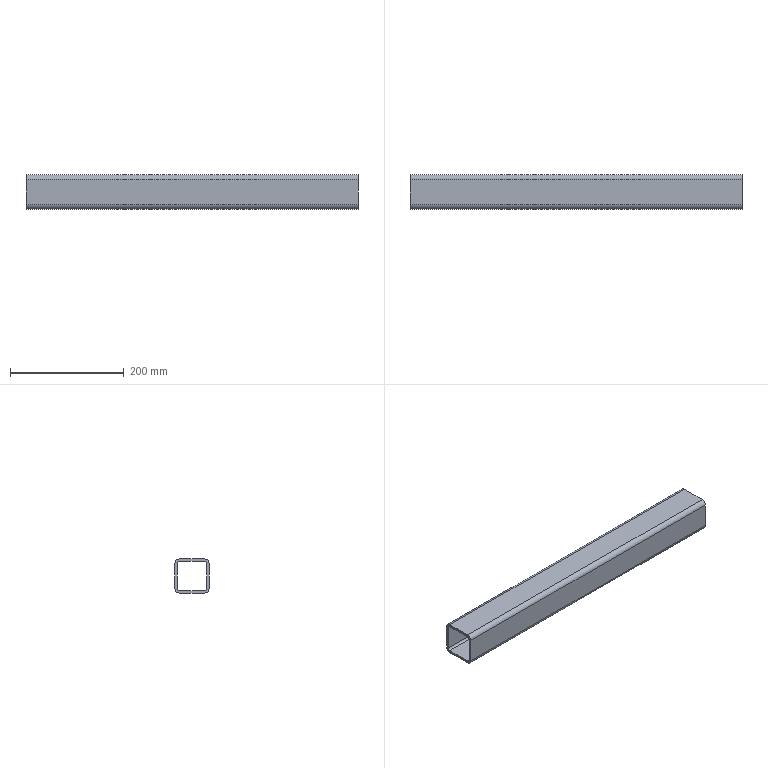Part | SolidWorks | features BaseBody 1 | 1 solid | 18 faces | box 585 x 60 x 60 mm | volume 500056 mm3 | plane 10 | cylinder 8 | commonest cylinder face diameters 8 x4 16 x4
STEP:
#1=CARTESIAN_POINT('',(-55.,2436.,-1248.));
#2=VERTEX_POINT('',#1);
#3=CARTESIAN_POINT('',(-55.,2436.,-1292.));
#4=VERTEX_POINT('',#3);
#5=CARTESIAN_POINT('',(-55.,2436.,-1248.));
#6=DIRECTION('',(0.,0.,-1.));
#7=VECTOR('',#6,1000.);
#8=LINE('',#5,#7);
#9=EDGE_CURVE('',#2,#4,#8,.T.);
#10=ORIENTED_EDGE('',*,*,#9,.T.);
#11=CARTESIAN_POINT('',(-640.,2436.,-1292.));
#12=VERTEX_POINT('',#11);
#13=CARTESIAN_POINT('',(-670.,2436.,-1292.));
#14=DIRECTION('',(-1.,0.,0.));
#15=VECTOR('',#14,1000.);
#16=LINE('',#13,#15);
#17=EDGE_CURVE('',#4,#12,#16,.T.);
#18=ORIENTED_EDGE('',*,*,#17,.T.);
#19=CARTESIAN_POINT('',(-640.,2436.,-1248.));
#20=VERTEX_POINT('',#19);
#21=CARTESIAN_POINT('',(-640.,2436.,-1248.));
#22=DIRECTION('',(0.,0.,1.));
#23=VECTOR('',#22,1000.);
#24=LINE('',#21,#23);
#25=EDGE_CURVE('',#12,#20,#24,.T.);
#26=ORIENTED_EDGE('',*,*,#25,.T.);
#27=CARTESIAN_POINT('',(-670.,2436.,-1248.));
#28=DIRECTION('',(1.,0.,0.));
#29=VECTOR('',#28,1000.);
#30=LINE('',#27,#29);
#31=EDGE_CURVE('',#20,#2,#30,.T.);
#32=ORIENTED_EDGE('',*,*,#31,.T.);
#33=EDGE_LOOP('',(#10,#18,#26,#32));
#34=FACE_OUTER_BOUND('',#33,.T.);
#35=CARTESIAN_POINT('',(-670.,2436.,-1248.));
#36=DIRECTION('',(0.,1.,0.));
#37=DIRECTION('',(0.,0.,1.));
#38=AXIS2_PLACEMENT_3D('',#35,#36,#37);
#39=PLANE('',#38);
#40=ADVANCED_FACE('',(#34),#39,.T.);
#41=ORIENTED_EDGE('',*,*,#17,.F.);
#42=CARTESIAN_POINT('',(-55.,2440.,-1296.));
#43=VERTEX_POINT('',#42);
#44=CARTESIAN_POINT('',(-55.,2440.,-1292.));
#45=DIRECTION('',(-1.,0.,0.));
#46=DIRECTION('',(0.,0.,-1.));
#47=AXIS2_PLACEMENT_3D('',#44,#45,#46);
#48=CIRCLE('',#47,4.);
#49=EDGE_CURVE('',#43,#4,#48,.T.);
#50=ORIENTED_EDGE('',*,*,#49,.F.);
#51=CARTESIAN_POINT('',(-640.,2440.,-1296.));
#52=VERTEX_POINT('',#51);
#53=CARTESIAN_POINT('',(-670.,2440.,-1296.));
#54=DIRECTION('',(1.,0.,0.));
#55=VECTOR('',#54,1000.);
#56=LINE('',#53,#55);
#57=EDGE_CURVE('',#52,#43,#56,.T.);
#58=ORIENTED_EDGE('',*,*,#57,.F.);
#59=CARTESIAN_POINT('',(-640.,2440.,-1292.));
#60=DIRECTION('',(1.,0.,0.));
#61=DIRECTION('',(0.,0.,-1.));
#62=AXIS2_PLACEMENT_3D('',#59,#60,#61);
#63=CIRCLE('',#62,4.);
#64=EDGE_CURVE('',#12,#52,#63,.T.);
#65=ORIENTED_EDGE('',*,*,#64,.F.);
#66=EDGE_LOOP('',(#41,#50,#58,#65));
#67=FACE_OUTER_BOUND('',#66,.T.);
#68=CARTESIAN_POINT('',(-670.,2440.,-1292.));
#69=DIRECTION('',(1.,0.,0.));
#70=DIRECTION('',(0.,0.,-1.));
#71=AXIS2_PLACEMENT_3D('',#68,#69,#70);
#72=CYLINDRICAL_SURFACE('',#71,4.);
#73=ADVANCED_FACE('',(#67),#72,.F.);
#74=CARTESIAN_POINT('',(-55.,2440.,-1244.));
#75=VERTEX_POINT('',#74);
#76=CARTESIAN_POINT('',(-55.,2440.,-1248.));
#77=DIRECTION('',(1.,0.,0.));
#78=DIRECTION('',(0.,0.,-1.));
#79=AXIS2_PLACEMENT_3D('',#76,#77,#78);
#80=CIRCLE('',#79,4.);
#81=EDGE_CURVE('',#75,#2,#80,.T.);
#82=ORIENTED_EDGE('',*,*,#81,.F.);
#83=CARTESIAN_POINT('',(-55.,2484.,-1244.));
#84=VERTEX_POINT('',#83);
#85=CARTESIAN_POINT('',(-55.,2462.,-1244.));
#86=DIRECTION('',(0.,-1.,0.));
#87=VECTOR('',#86,1000.);
#88=LINE('',#85,#87);
#89=EDGE_CURVE('',#84,#75,#88,.T.);
#90=ORIENTED_EDGE('',*,*,#89,.F.);
#91=CARTESIAN_POINT('',(-55.,2488.,-1248.));
#92=VERTEX_POINT('',#91);
#93=CARTESIAN_POINT('',(-55.,2484.,-1248.));
#94=DIRECTION('',(1.,0.,0.));
#95=DIRECTION('',(0.,0.,-1.));
#96=AXIS2_PLACEMENT_3D('',#93,#94,#95);
#97=CIRCLE('',#96,4.);
#98=EDGE_CURVE('',#92,#84,#97,.T.);
#99=ORIENTED_EDGE('',*,*,#98,.F.);
#100=CARTESIAN_POINT('',(-55.,2488.,-1292.));
#101=VERTEX_POINT('',#100);
#102=CARTESIAN_POINT('',(-55.,2488.,-400.));
#103=DIRECTION('',(0.,0.,1.));
#104=VECTOR('',#103,1000.);
#105=LINE('',#102,#104);
#106=EDGE_CURVE('',#101,#92,#105,.T.);
#107=ORIENTED_EDGE('',*,*,#106,.F.);
#108=CARTESIAN_POINT('',(-55.,2484.,-1296.));
#109=VERTEX_POINT('',#108);
#110=CARTESIAN_POINT('',(-55.,2484.,-1292.));
#111=DIRECTION('',(1.,0.,0.));
#112=DIRECTION('',(0.,0.,-1.));
#113=AXIS2_PLACEMENT_3D('',#110,#111,#112);
#114=CIRCLE('',#113,4.);
#115=EDGE_CURVE('',#109,#101,#114,.T.);
#116=ORIENTED_EDGE('',*,*,#115,.F.);
#117=CARTESIAN_POINT('',(-55.,2462.,-1296.));
#118=DIRECTION('',(0.,1.,0.));
#119=VECTOR('',#118,1000.);
#120=LINE('',#117,#119);
#121=EDGE_CURVE('',#43,#109,#120,.T.);
#122=ORIENTED_EDGE('',*,*,#121,.F.);
#123=ORIENTED_EDGE('',*,*,#49,.T.);
#124=ORIENTED_EDGE('',*,*,#9,.F.);
#125=EDGE_LOOP('',(#82,#90,#99,#107,#116,#122,#123,#124));
#126=FACE_BOUND('',#125,.T.);
#127=CARTESIAN_POINT('',(-55.,2440.,-1240.));
#128=VERTEX_POINT('',#127);
#129=CARTESIAN_POINT('',(-55.,2484.,-1240.));
#130=VERTEX_POINT('',#129);
#131=CARTESIAN_POINT('',(-55.,2462.,-1240.));
#132=DIRECTION('',(0.,1.,0.));
#133=VECTOR('',#132,1000.);
#134=LINE('',#131,#133);
#135=EDGE_CURVE('',#128,#130,#134,.T.);
#136=ORIENTED_EDGE('',*,*,#135,.F.);
#137=CARTESIAN_POINT('',(-55.,2432.,-1248.));
#138=VERTEX_POINT('',#137);
#139=CARTESIAN_POINT('',(-55.,2440.,-1248.));
#140=DIRECTION('',(-1.,0.,0.));
#141=DIRECTION('',(0.,0.,-1.));
#142=AXIS2_PLACEMENT_3D('',#139,#140,#141);
#143=CIRCLE('',#142,8.);
#144=EDGE_CURVE('',#138,#128,#143,.T.);
#145=ORIENTED_EDGE('',*,*,#144,.F.);
#146=CARTESIAN_POINT('',(-55.,2432.,-1292.));
#147=VERTEX_POINT('',#146);
#148=CARTESIAN_POINT('',(-55.,2432.,-400.));
#149=DIRECTION('',(0.,0.,1.));
#150=VECTOR('',#149,1000.);
#151=LINE('',#148,#150);
#152=EDGE_CURVE('',#147,#138,#151,.T.);
#153=ORIENTED_EDGE('',*,*,#152,.F.);
#154=CARTESIAN_POINT('',(-55.,2440.,-1300.));
#155=VERTEX_POINT('',#154);
#156=CARTESIAN_POINT('',(-55.,2440.,-1292.));
#157=DIRECTION('',(-1.,0.,0.));
#158=DIRECTION('',(0.,0.,-1.));
#159=AXIS2_PLACEMENT_3D('',#156,#157,#158);
#160=CIRCLE('',#159,8.);
#161=EDGE_CURVE('',#155,#147,#160,.T.);
#162=ORIENTED_EDGE('',*,*,#161,.F.);
#163=CARTESIAN_POINT('',(-55.,2484.,-1300.));
#164=VERTEX_POINT('',#163);
#165=CARTESIAN_POINT('',(-55.,2462.,-1300.));
#166=DIRECTION('',(0.,-1.,0.));
#167=VECTOR('',#166,1000.);
#168=LINE('',#165,#167);
#169=EDGE_CURVE('',#164,#155,#168,.T.);
#170=ORIENTED_EDGE('',*,*,#169,.F.);
#171=CARTESIAN_POINT('',(-55.,2492.,-1292.));
#172=VERTEX_POINT('',#171);
#173=CARTESIAN_POINT('',(-55.,2484.,-1292.));
#174=DIRECTION('',(-1.,0.,0.));
#175=DIRECTION('',(0.,0.,-1.));
#176=AXIS2_PLACEMENT_3D('',#173,#174,#175);
#177=CIRCLE('',#176,8.);
#178=EDGE_CURVE('',#172,#164,#177,.T.);
#179=ORIENTED_EDGE('',*,*,#178,.F.);
#180=CARTESIAN_POINT('',(-55.,2492.,-1248.));
#181=VERTEX_POINT('',#180);
#182=CARTESIAN_POINT('',(-55.,2492.,-400.));
#183=DIRECTION('',(0.,0.,-1.));
#184=VECTOR('',#183,1000.);
#185=LINE('',#182,#184);
#186=EDGE_CURVE('',#181,#172,#185,.T.);
#187=ORIENTED_EDGE('',*,*,#186,.F.);
#188=CARTESIAN_POINT('',(-55.,2484.,-1248.));
#189=DIRECTION('',(-1.,0.,0.));
#190=DIRECTION('',(0.,0.,-1.));
#191=AXIS2_PLACEMENT_3D('',#188,#189,#190);
#192=CIRCLE('',#191,8.);
#193=EDGE_CURVE('',#130,#181,#192,.T.);
#194=ORIENTED_EDGE('',*,*,#193,.F.);
#195=EDGE_LOOP('',(#136,#145,#153,#162,#170,#179,#187,#194));
#196=FACE_OUTER_BOUND('',#195,.T.);
#197=CARTESIAN_POINT('',(-55.,2462.,-400.));
#198=DIRECTION('',(-1.,0.,0.));
#199=DIRECTION('',(0.,0.,1.));
#200=AXIS2_PLACEMENT_3D('',#197,#198,#199);
#201=PLANE('',#200);
#202=ADVANCED_FACE('',(#126,#196),#201,.F.);
#203=CARTESIAN_POINT('',(-640.,2440.,-1244.));
#204=VERTEX_POINT('',#203);
#205=CARTESIAN_POINT('',(-670.,2440.,-1244.));
#206=DIRECTION('',(-1.,0.,0.));
#207=VECTOR('',#206,1000.);
#208=LINE('',#205,#207);
#209=EDGE_CURVE('',#75,#204,#208,.T.);
#210=ORIENTED_EDGE('',*,*,#209,.F.);
#211=ORIENTED_EDGE('',*,*,#81,.T.);
#212=ORIENTED_EDGE('',*,*,#31,.F.);
#213=CARTESIAN_POINT('',(-640.,2440.,-1248.));
#214=DIRECTION('',(1.,0.,0.));
#215=DIRECTION('',(0.,0.,-1.));
#216=AXIS2_PLACEMENT_3D('',#213,#214,#215);
#217=CIRCLE('',#216,4.);
#218=EDGE_CURVE('',#204,#20,#217,.T.);
#219=ORIENTED_EDGE('',*,*,#218,.F.);
#220=EDGE_LOOP('',(#210,#211,#212,#219));
#221=FACE_OUTER_BOUND('',#220,.T.);
#222=CARTESIAN_POINT('',(-670.,2440.,-1248.));
#223=DIRECTION('',(1.,0.,0.));
#224=DIRECTION('',(0.,0.,-1.));
#225=AXIS2_PLACEMENT_3D('',#222,#223,#224);
#226=CYLINDRICAL_SURFACE('',#225,4.);
#227=ADVANCED_FACE('',(#221),#226,.F.);
#228=ORIENTED_EDGE('',*,*,#64,.T.);
#229=CARTESIAN_POINT('',(-640.,2484.,-1296.));
#230=VERTEX_POINT('',#229);
#231=CARTESIAN_POINT('',(-640.,1242.,-1296.));
#232=DIRECTION('',(0.,1.,0.));
#233=VECTOR('',#232,1000.);
#234=LINE('',#231,#233);
#235=EDGE_CURVE('',#52,#230,#234,.T.);
#236=ORIENTED_EDGE('',*,*,#235,.T.);
#237=CARTESIAN_POINT('',(-640.,2488.,-1292.));
#238=VERTEX_POINT('',#237);
#239=CARTESIAN_POINT('',(-640.,2484.,-1292.));
#240=DIRECTION('',(1.,0.,0.));
#241=DIRECTION('',(0.,0.,-1.));
#242=AXIS2_PLACEMENT_3D('',#239,#240,#241);
#243=CIRCLE('',#242,4.);
#244=EDGE_CURVE('',#230,#238,#243,.T.);
#245=ORIENTED_EDGE('',*,*,#244,.T.);
#246=CARTESIAN_POINT('',(-640.,2488.,-1248.));
#247=VERTEX_POINT('',#246);
#248=CARTESIAN_POINT('',(-640.,2488.,-1248.));
#249=DIRECTION('',(0.,0.,1.));
#250=VECTOR('',#249,1000.);
#251=LINE('',#248,#250);
#252=EDGE_CURVE('',#238,#247,#251,.T.);
#253=ORIENTED_EDGE('',*,*,#252,.T.);
#254=CARTESIAN_POINT('',(-640.,2484.,-1244.));
#255=VERTEX_POINT('',#254);
#256=CARTESIAN_POINT('',(-640.,2484.,-1248.));
#257=DIRECTION('',(1.,0.,0.));
#258=DIRECTION('',(0.,0.,-1.));
#259=AXIS2_PLACEMENT_3D('',#256,#257,#258);
#260=CIRCLE('',#259,4.);
#261=EDGE_CURVE('',#247,#255,#260,.T.);
#262=ORIENTED_EDGE('',*,*,#261,.T.);
#263=CARTESIAN_POINT('',(-640.,1242.,-1244.));
#264=DIRECTION('',(0.,-1.,0.));
#265=VECTOR('',#264,1000.);
#266=LINE('',#263,#265);
#267=EDGE_CURVE('',#255,#204,#266,.T.);
#268=ORIENTED_EDGE('',*,*,#267,.T.);
#269=ORIENTED_EDGE('',*,*,#218,.T.);
#270=ORIENTED_EDGE('',*,*,#25,.F.);
#271=EDGE_LOOP('',(#228,#236,#245,#253,#262,#268,#269,#270));
#272=FACE_BOUND('',#271,.T.);
#273=CARTESIAN_POINT('',(-640.,2484.,-1300.));
#274=VERTEX_POINT('',#273);
#275=CARTESIAN_POINT('',(-640.,2440.,-1300.));
#276=VERTEX_POINT('',#275);
#277=CARTESIAN_POINT('',(-640.,1242.,-1300.));
#278=DIRECTION('',(0.,-1.,0.));
#279=VECTOR('',#278,1000.);
#280=LINE('',#277,#279);
#281=EDGE_CURVE('',#274,#276,#280,.T.);
#282=ORIENTED_EDGE('',*,*,#281,.T.);
#283=CARTESIAN_POINT('',(-640.,2432.,-1292.));
#284=VERTEX_POINT('',#283);
#285=CARTESIAN_POINT('',(-640.,2440.,-1292.));
#286=DIRECTION('',(-1.,0.,0.));
#287=DIRECTION('',(0.,0.,-1.));
#288=AXIS2_PLACEMENT_3D('',#285,#286,#287);
#289=CIRCLE('',#288,8.);
#290=EDGE_CURVE('',#276,#284,#289,.T.);
#291=ORIENTED_EDGE('',*,*,#290,.T.);
#292=CARTESIAN_POINT('',(-640.,2432.,-1248.));
#293=VERTEX_POINT('',#292);
#294=CARTESIAN_POINT('',(-640.,2432.,-1248.));
#295=DIRECTION('',(0.,0.,1.));
#296=VECTOR('',#295,1000.);
#297=LINE('',#294,#296);
#298=EDGE_CURVE('',#284,#293,#297,.T.);
#299=ORIENTED_EDGE('',*,*,#298,.T.);
#300=CARTESIAN_POINT('',(-640.,2440.,-1240.));
#301=VERTEX_POINT('',#300);
#302=CARTESIAN_POINT('',(-640.,2440.,-1248.));
#303=DIRECTION('',(-1.,0.,0.));
#304=DIRECTION('',(0.,0.,-1.));
#305=AXIS2_PLACEMENT_3D('',#302,#303,#304);
#306=CIRCLE('',#305,8.);
#307=EDGE_CURVE('',#293,#301,#306,.T.);
#308=ORIENTED_EDGE('',*,*,#307,.T.);
#309=CARTESIAN_POINT('',(-640.,2484.,-1240.));
#310=VERTEX_POINT('',#309);
#311=CARTESIAN_POINT('',(-640.,1242.,-1240.));
#312=DIRECTION('',(0.,1.,0.));
#313=VECTOR('',#312,1000.);
#314=LINE('',#311,#313);
#315=EDGE_CURVE('',#301,#310,#314,.T.);
#316=ORIENTED_EDGE('',*,*,#315,.T.);
#317=CARTESIAN_POINT('',(-640.,2492.,-1248.));
#318=VERTEX_POINT('',#317);
#319=CARTESIAN_POINT('',(-640.,2484.,-1248.));
#320=DIRECTION('',(-1.,0.,0.));
#321=DIRECTION('',(0.,0.,-1.));
#322=AXIS2_PLACEMENT_3D('',#319,#320,#321);
#323=CIRCLE('',#322,8.);
#324=EDGE_CURVE('',#310,#318,#323,.T.);
#325=ORIENTED_EDGE('',*,*,#324,.T.);
#326=CARTESIAN_POINT('',(-640.,2492.,-1292.));
#327=VERTEX_POINT('',#326);
#328=CARTESIAN_POINT('',(-640.,2492.,-1248.));
#329=DIRECTION('',(0.,0.,-1.));
#330=VECTOR('',#329,1000.);
#331=LINE('',#328,#330);
#332=EDGE_CURVE('',#318,#327,#331,.T.);
#333=ORIENTED_EDGE('',*,*,#332,.T.);
#334=CARTESIAN_POINT('',(-640.,2484.,-1292.));
#335=DIRECTION('',(-1.,0.,0.));
#336=DIRECTION('',(0.,0.,-1.));
#337=AXIS2_PLACEMENT_3D('',#334,#335,#336);
#338=CIRCLE('',#337,8.);
#339=EDGE_CURVE('',#327,#274,#338,.T.);
#340=ORIENTED_EDGE('',*,*,#339,.T.);
#341=EDGE_LOOP('',(#282,#291,#299,#308,#316,#325,#333,#340));
#342=FACE_OUTER_BOUND('',#341,.T.);
#343=CARTESIAN_POINT('',(-640.,1242.,-1248.));
#344=DIRECTION('',(-1.,0.,0.));
#345=DIRECTION('',(0.,0.,1.));
#346=AXIS2_PLACEMENT_3D('',#343,#344,#345);
#347=PLANE('',#346);
#348=ADVANCED_FACE('',(#272,#342),#347,.T.);
#349=ORIENTED_EDGE('',*,*,#121,.T.);
#350=CARTESIAN_POINT('',(-670.,2484.,-1296.));
#351=DIRECTION('',(-1.,0.,0.));
#352=VECTOR('',#351,1000.);
#353=LINE('',#350,#352);
#354=EDGE_CURVE('',#109,#230,#353,.T.);
#355=ORIENTED_EDGE('',*,*,#354,.T.);
#356=ORIENTED_EDGE('',*,*,#235,.F.);
#357=ORIENTED_EDGE('',*,*,#57,.T.);
#358=EDGE_LOOP('',(#349,#355,#356,#357));
#359=FACE_OUTER_BOUND('',#358,.T.);
#360=CARTESIAN_POINT('',(-670.,2484.,-1296.));
#361=DIRECTION('',(0.,0.,1.));
#362=DIRECTION('',(1.,0.,0.));
#363=AXIS2_PLACEMENT_3D('',#360,#361,#362);
#364=PLANE('',#363);
#365=ADVANCED_FACE('',(#359),#364,.T.);
#366=ORIENTED_EDGE('',*,*,#89,.T.);
#367=ORIENTED_EDGE('',*,*,#209,.T.);
#368=ORIENTED_EDGE('',*,*,#267,.F.);
#369=CARTESIAN_POINT('',(-670.,2484.,-1244.));
#370=DIRECTION('',(1.,0.,0.));
#371=VECTOR('',#370,1000.);
#372=LINE('',#369,#371);
#373=EDGE_CURVE('',#255,#84,#372,.T.);
#374=ORIENTED_EDGE('',*,*,#373,.T.);
#375=EDGE_LOOP('',(#366,#367,#368,#374));
#376=FACE_OUTER_BOUND('',#375,.T.);
#377=CARTESIAN_POINT('',(-670.,2440.,-1244.));
#378=DIRECTION('',(0.,0.,-1.));
#379=DIRECTION('',(-1.,0.,0.));
#380=AXIS2_PLACEMENT_3D('',#377,#378,#379);
#381=PLANE('',#380);
#382=ADVANCED_FACE('',(#376),#381,.T.);
#383=CARTESIAN_POINT('',(-670.,2488.,-1248.));
#384=DIRECTION('',(-1.,0.,0.));
#385=VECTOR('',#384,1000.);
#386=LINE('',#383,#385);
#387=EDGE_CURVE('',#92,#247,#386,.T.);
#388=ORIENTED_EDGE('',*,*,#387,.F.);
#389=ORIENTED_EDGE('',*,*,#98,.T.);
#390=ORIENTED_EDGE('',*,*,#373,.F.);
#391=ORIENTED_EDGE('',*,*,#261,.F.);
#392=EDGE_LOOP('',(#388,#389,#390,#391));
#393=FACE_OUTER_BOUND('',#392,.T.);
#394=CARTESIAN_POINT('',(-670.,2484.,-1248.));
#395=DIRECTION('',(1.,0.,0.));
#396=DIRECTION('',(0.,0.,-1.));
#397=AXIS2_PLACEMENT_3D('',#394,#395,#396);
#398=CYLINDRICAL_SURFACE('',#397,4.);
#399=ADVANCED_FACE('',(#393),#398,.F.);
#400=ORIENTED_EDGE('',*,*,#106,.T.);
#401=ORIENTED_EDGE('',*,*,#387,.T.);
#402=ORIENTED_EDGE('',*,*,#252,.F.);
#403=CARTESIAN_POINT('',(-670.,2488.,-1292.));
#404=DIRECTION('',(1.,0.,0.));
#405=VECTOR('',#404,1000.);
#406=LINE('',#403,#405);
#407=EDGE_CURVE('',#238,#101,#406,.T.);
#408=ORIENTED_EDGE('',*,*,#407,.T.);
#409=EDGE_LOOP('',(#400,#401,#402,#408));
#410=FACE_OUTER_BOUND('',#409,.T.);
#411=CARTESIAN_POINT('',(-670.,2488.,-1292.));
#412=DIRECTION('',(0.,-1.,0.));
#413=DIRECTION('',(0.,0.,-1.));
#414=AXIS2_PLACEMENT_3D('',#411,#412,#413);
#415=PLANE('',#414);
#416=ADVANCED_FACE('',(#410),#415,.T.);
#417=ORIENTED_EDGE('',*,*,#354,.F.);
#418=ORIENTED_EDGE('',*,*,#115,.T.);
#419=ORIENTED_EDGE('',*,*,#407,.F.);
#420=ORIENTED_EDGE('',*,*,#244,.F.);
#421=EDGE_LOOP('',(#417,#418,#419,#420));
#422=FACE_OUTER_BOUND('',#421,.T.);
#423=CARTESIAN_POINT('',(-670.,2484.,-1292.));
#424=DIRECTION('',(1.,0.,0.));
#425=DIRECTION('',(0.,0.,-1.));
#426=AXIS2_PLACEMENT_3D('',#423,#424,#425);
#427=CYLINDRICAL_SURFACE('',#426,4.);
#428=ADVANCED_FACE('',(#422),#427,.F.);
#429=CARTESIAN_POINT('',(-670.,2492.,-1248.));
#430=DIRECTION('',(-1.,0.,0.));
#431=VECTOR('',#430,1000.);
#432=LINE('',#429,#431);
#433=EDGE_CURVE('',#181,#318,#432,.T.);
#434=ORIENTED_EDGE('',*,*,#433,.T.);
#435=ORIENTED_EDGE('',*,*,#324,.F.);
#436=CARTESIAN_POINT('',(-670.,2484.,-1240.));
#437=DIRECTION('',(1.,0.,0.));
#438=VECTOR('',#437,1000.);
#439=LINE('',#436,#438);
#440=EDGE_CURVE('',#310,#130,#439,.T.);
#441=ORIENTED_EDGE('',*,*,#440,.T.);
#442=ORIENTED_EDGE('',*,*,#193,.T.);
#443=EDGE_LOOP('',(#434,#435,#441,#442));
#444=FACE_OUTER_BOUND('',#443,.T.);
#445=CARTESIAN_POINT('',(-670.,2484.,-1248.));
#446=DIRECTION('',(1.,0.,0.));
#447=DIRECTION('',(0.,0.,-1.));
#448=AXIS2_PLACEMENT_3D('',#445,#446,#447);
#449=CYLINDRICAL_SURFACE('',#448,8.);
#450=ADVANCED_FACE('',(#444),#449,.T.);
#451=ORIENTED_EDGE('',*,*,#135,.T.);
#452=ORIENTED_EDGE('',*,*,#440,.F.);
#453=ORIENTED_EDGE('',*,*,#315,.F.);
#454=CARTESIAN_POINT('',(-670.,2440.,-1240.));
#455=DIRECTION('',(-1.,0.,0.));
#456=VECTOR('',#455,1000.);
#457=LINE('',#454,#456);
#458=EDGE_CURVE('',#128,#301,#457,.T.);
#459=ORIENTED_EDGE('',*,*,#458,.F.);
#460=EDGE_LOOP('',(#451,#452,#453,#459));
#461=FACE_OUTER_BOUND('',#460,.T.);
#462=CARTESIAN_POINT('',(-670.,2440.,-1240.));
#463=DIRECTION('',(0.,0.,-1.));
#464=DIRECTION('',(-1.,0.,0.));
#465=AXIS2_PLACEMENT_3D('',#462,#463,#464);
#466=PLANE('',#465);
#467=ADVANCED_FACE('',(#461),#466,.F.);
#468=ORIENTED_EDGE('',*,*,#458,.T.);
#469=ORIENTED_EDGE('',*,*,#307,.F.);
#470=CARTESIAN_POINT('',(-670.,2432.,-1248.));
#471=DIRECTION('',(1.,0.,0.));
#472=VECTOR('',#471,1000.);
#473=LINE('',#470,#472);
#474=EDGE_CURVE('',#293,#138,#473,.T.);
#475=ORIENTED_EDGE('',*,*,#474,.T.);
#476=ORIENTED_EDGE('',*,*,#144,.T.);
#477=EDGE_LOOP('',(#468,#469,#475,#476));
#478=FACE_OUTER_BOUND('',#477,.T.);
#479=CARTESIAN_POINT('',(-670.,2440.,-1248.));
#480=DIRECTION('',(1.,0.,0.));
#481=DIRECTION('',(0.,0.,-1.));
#482=AXIS2_PLACEMENT_3D('',#479,#480,#481);
#483=CYLINDRICAL_SURFACE('',#482,8.);
#484=ADVANCED_FACE('',(#478),#483,.T.);
#485=ORIENTED_EDGE('',*,*,#152,.T.);
#486=ORIENTED_EDGE('',*,*,#474,.F.);
#487=ORIENTED_EDGE('',*,*,#298,.F.);
#488=CARTESIAN_POINT('',(-670.,2432.,-1292.));
#489=DIRECTION('',(-1.,0.,0.));
#490=VECTOR('',#489,1000.);
#491=LINE('',#488,#490);
#492=EDGE_CURVE('',#147,#284,#491,.T.);
#493=ORIENTED_EDGE('',*,*,#492,.F.);
#494=EDGE_LOOP('',(#485,#486,#487,#493));
#495=FACE_OUTER_BOUND('',#494,.T.);
#496=CARTESIAN_POINT('',(-670.,2432.,-1248.));
#497=DIRECTION('',(0.,1.,0.));
#498=DIRECTION('',(0.,0.,1.));
#499=AXIS2_PLACEMENT_3D('',#496,#497,#498);
#500=PLANE('',#499);
#501=ADVANCED_FACE('',(#495),#500,.F.);
#502=ORIENTED_EDGE('',*,*,#492,.T.);
#503=ORIENTED_EDGE('',*,*,#290,.F.);
#504=CARTESIAN_POINT('',(-670.,2440.,-1300.));
#505=DIRECTION('',(1.,0.,0.));
#506=VECTOR('',#505,1000.);
#507=LINE('',#504,#506);
#508=EDGE_CURVE('',#276,#155,#507,.T.);
#509=ORIENTED_EDGE('',*,*,#508,.T.);
#510=ORIENTED_EDGE('',*,*,#161,.T.);
#511=EDGE_LOOP('',(#502,#503,#509,#510));
#512=FACE_OUTER_BOUND('',#511,.T.);
#513=CARTESIAN_POINT('',(-670.,2440.,-1292.));
#514=DIRECTION('',(1.,0.,0.));
#515=DIRECTION('',(0.,0.,-1.));
#516=AXIS2_PLACEMENT_3D('',#513,#514,#515);
#517=CYLINDRICAL_SURFACE('',#516,8.);
#518=ADVANCED_FACE('',(#512),#517,.T.);
#519=ORIENTED_EDGE('',*,*,#169,.T.);
#520=ORIENTED_EDGE('',*,*,#508,.F.);
#521=ORIENTED_EDGE('',*,*,#281,.F.);
#522=CARTESIAN_POINT('',(-670.,2484.,-1300.));
#523=DIRECTION('',(-1.,0.,0.));
#524=VECTOR('',#523,1000.);
#525=LINE('',#522,#524);
#526=EDGE_CURVE('',#164,#274,#525,.T.);
#527=ORIENTED_EDGE('',*,*,#526,.F.);
#528=EDGE_LOOP('',(#519,#520,#521,#527));
#529=FACE_OUTER_BOUND('',#528,.T.);
#530=CARTESIAN_POINT('',(-670.,2484.,-1300.));
#531=DIRECTION('',(0.,0.,1.));
#532=DIRECTION('',(1.,0.,0.));
#533=AXIS2_PLACEMENT_3D('',#530,#531,#532);
#534=PLANE('',#533);
#535=ADVANCED_FACE('',(#529),#534,.F.);
#536=ORIENTED_EDGE('',*,*,#526,.T.);
#537=ORIENTED_EDGE('',*,*,#339,.F.);
#538=CARTESIAN_POINT('',(-670.,2492.,-1292.));
#539=DIRECTION('',(1.,0.,0.));
#540=VECTOR('',#539,1000.);
#541=LINE('',#538,#540);
#542=EDGE_CURVE('',#327,#172,#541,.T.);
#543=ORIENTED_EDGE('',*,*,#542,.T.);
#544=ORIENTED_EDGE('',*,*,#178,.T.);
#545=EDGE_LOOP('',(#536,#537,#543,#544));
#546=FACE_OUTER_BOUND('',#545,.T.);
#547=CARTESIAN_POINT('',(-670.,2484.,-1292.));
#548=DIRECTION('',(1.,0.,0.));
#549=DIRECTION('',(0.,0.,-1.));
#550=AXIS2_PLACEMENT_3D('',#547,#548,#549);
#551=CYLINDRICAL_SURFACE('',#550,8.);
#552=ADVANCED_FACE('',(#546),#551,.T.);
#553=ORIENTED_EDGE('',*,*,#186,.T.);
#554=ORIENTED_EDGE('',*,*,#542,.F.);
#555=ORIENTED_EDGE('',*,*,#332,.F.);
#556=ORIENTED_EDGE('',*,*,#433,.F.);
#557=EDGE_LOOP('',(#553,#554,#555,#556));
#558=FACE_OUTER_BOUND('',#557,.T.);
#559=CARTESIAN_POINT('',(-670.,2492.,-1292.));
#560=DIRECTION('',(0.,-1.,0.));
#561=DIRECTION('',(0.,0.,-1.));
#562=AXIS2_PLACEMENT_3D('',#559,#560,#561);
#563=PLANE('',#562);
#564=ADVANCED_FACE('',(#558),#563,.F.);
#565=CLOSED_SHELL('',(#40,#73,#202,#227,#348,#365,#382,#399,#416,#428,#450,#467,#484,#501,#518,#535,#552,#564));
#566=MANIFOLD_SOLID_BREP('',#565);
#567=CARTESIAN_POINT('',(0.,0.,0.));
#568=DIRECTION('',(0.,0.,1.));
#569=DIRECTION('',(1.,0.,0.));
#570=AXIS2_PLACEMENT_3D('',#567,#568,#569);
#571=(LENGTH_UNIT()NAMED_UNIT(*)SI_UNIT(.MILLI.,.METRE.));
#572=UNCERTAINTY_MEASURE_WITH_UNIT(LENGTH_MEASURE(0.00001),#571,'','');
#573=(NAMED_UNIT(*)PLANE_ANGLE_UNIT()SI_UNIT($,.RADIAN.));
#574=(NAMED_UNIT(*)SI_UNIT($,.STERADIAN.)SOLID_ANGLE_UNIT());
#575=(GEOMETRIC_REPRESENTATION_CONTEXT(3)GLOBAL_UNCERTAINTY_ASSIGNED_CONTEXT((#572))GLOBAL_UNIT_ASSIGNED_CONTEXT((#571,#573,#574))REPRESENTATION_CONTEXT('',''));
#576=ADVANCED_BREP_SHAPE_REPRESENTATION('',(#566,#570),#575);